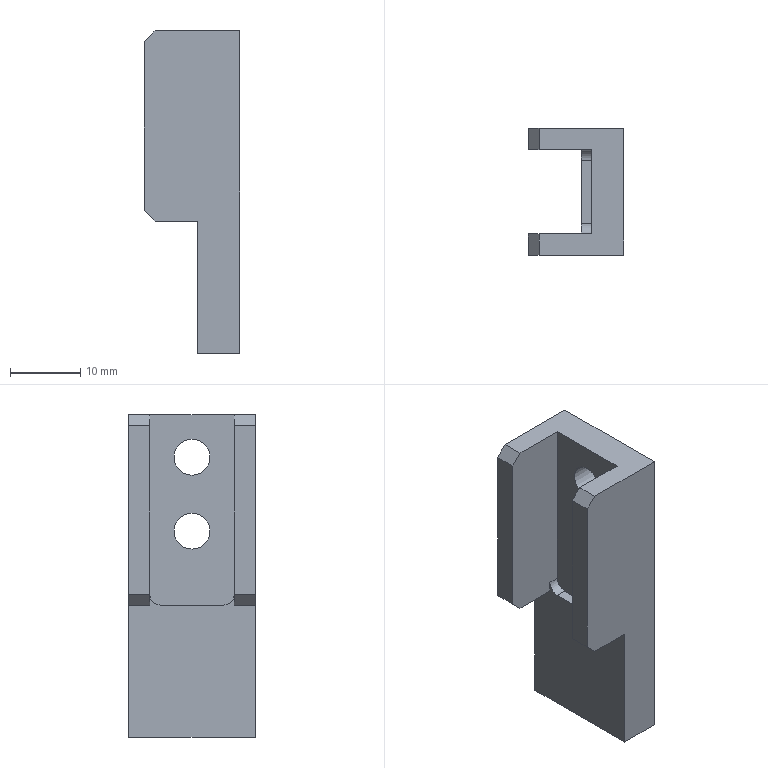Part | NX | features 倒角2 2 | 1 solid | 24 faces | box 13.5 x 18 x 45.75 mm | volume 5474 mm3 | plane 18 | cylinder 6 | commonest cylinder face diameters 5.1 x4 3 x2
STEP:
#1=CARTESIAN_POINT('',(126.798,-42.7,-33.95));
#2=VERTEX_POINT('',#1);
#3=CARTESIAN_POINT('',(126.798,-42.7,-39.05));
#4=VERTEX_POINT('',#3);
#5=CARTESIAN_POINT('',(126.798,-42.7,-36.5));
#6=DIRECTION('',(-1.,0.,0.));
#7=DIRECTION('',(0.,0.,1.));
#8=AXIS2_PLACEMENT_3D('',#5,#6,#7);
#9=CIRCLE('',#8,2.55);
#10=EDGE_CURVE('',#2,#4,#9,.F.);
#11=ORIENTED_EDGE('',*,*,#10,.F.);
#12=CARTESIAN_POINT('',(131.298,-42.7,-33.95));
#13=VERTEX_POINT('',#12);
#14=CARTESIAN_POINT('',(131.298,-42.7,-33.95));
#15=DIRECTION('',(1.,0.,0.));
#16=VECTOR('',#15,1000.);
#17=LINE('',#14,#16);
#18=EDGE_CURVE('',#13,#2,#17,.F.);
#19=ORIENTED_EDGE('',*,*,#18,.F.);
#20=CARTESIAN_POINT('',(131.298,-42.7,-39.05));
#21=VERTEX_POINT('',#20);
#22=CARTESIAN_POINT('',(131.298,-42.7,-36.5));
#23=DIRECTION('',(-1.,0.,0.));
#24=DIRECTION('',(0.,0.,1.));
#25=AXIS2_PLACEMENT_3D('',#22,#23,#24);
#26=CIRCLE('',#25,2.55);
#27=EDGE_CURVE('',#13,#21,#26,.F.);
#28=ORIENTED_EDGE('',*,*,#27,.T.);
#29=CARTESIAN_POINT('',(131.298,-42.7,-39.05));
#30=DIRECTION('',(1.,0.,0.));
#31=VECTOR('',#30,1000.);
#32=LINE('',#29,#31);
#33=EDGE_CURVE('',#4,#21,#32,.T.);
#34=ORIENTED_EDGE('',*,*,#33,.F.);
#35=EDGE_LOOP('',(#11,#19,#28,#34));
#36=FACE_BOUND('',#35,.T.);
#37=CARTESIAN_POINT('',(131.298,-42.7,-36.5));
#38=DIRECTION('',(1.,0.,0.));
#39=DIRECTION('',(0.,0.,-1.));
#40=AXIS2_PLACEMENT_3D('',#37,#38,#39);
#41=CYLINDRICAL_SURFACE('',#40,2.55);
#42=ADVANCED_FACE('',(#36),#41,.F.);
#43=CARTESIAN_POINT('',(126.798,-42.7,-23.45));
#44=VERTEX_POINT('',#43);
#45=CARTESIAN_POINT('',(126.798,-42.7,-28.55));
#46=VERTEX_POINT('',#45);
#47=CARTESIAN_POINT('',(126.798,-42.7,-26.));
#48=DIRECTION('',(-1.,0.,0.));
#49=DIRECTION('',(0.,0.,1.));
#50=AXIS2_PLACEMENT_3D('',#47,#48,#49);
#51=CIRCLE('',#50,2.55);
#52=EDGE_CURVE('',#44,#46,#51,.F.);
#53=ORIENTED_EDGE('',*,*,#52,.F.);
#54=CARTESIAN_POINT('',(131.298,-42.7,-23.45));
#55=VERTEX_POINT('',#54);
#56=CARTESIAN_POINT('',(131.298,-42.7,-23.45));
#57=DIRECTION('',(1.,0.,0.));
#58=VECTOR('',#57,1000.);
#59=LINE('',#56,#58);
#60=EDGE_CURVE('',#55,#44,#59,.F.);
#61=ORIENTED_EDGE('',*,*,#60,.F.);
#62=CARTESIAN_POINT('',(131.298,-42.7,-28.55));
#63=VERTEX_POINT('',#62);
#64=CARTESIAN_POINT('',(131.298,-42.7,-26.));
#65=DIRECTION('',(-1.,0.,0.));
#66=DIRECTION('',(0.,0.,1.));
#67=AXIS2_PLACEMENT_3D('',#64,#65,#66);
#68=CIRCLE('',#67,2.55);
#69=EDGE_CURVE('',#55,#63,#68,.F.);
#70=ORIENTED_EDGE('',*,*,#69,.T.);
#71=CARTESIAN_POINT('',(131.298,-42.7,-28.55));
#72=DIRECTION('',(1.,0.,0.));
#73=VECTOR('',#72,1000.);
#74=LINE('',#71,#73);
#75=EDGE_CURVE('',#46,#63,#74,.T.);
#76=ORIENTED_EDGE('',*,*,#75,.F.);
#77=EDGE_LOOP('',(#53,#61,#70,#76));
#78=FACE_BOUND('',#77,.T.);
#79=CARTESIAN_POINT('',(131.298,-42.7,-26.));
#80=DIRECTION('',(1.,0.,0.));
#81=DIRECTION('',(0.,0.,-1.));
#82=AXIS2_PLACEMENT_3D('',#79,#80,#81);
#83=CYLINDRICAL_SURFACE('',#82,2.55);
#84=ADVANCED_FACE('',(#78),#83,.F.);
#85=CARTESIAN_POINT('',(117.798,-33.7,-45.5));
#86=VERTEX_POINT('',#85);
#87=CARTESIAN_POINT('',(117.798,-33.7,-21.5));
#88=VERTEX_POINT('',#87);
#89=CARTESIAN_POINT('',(117.798,-33.7,-42.5));
#90=DIRECTION('',(0.,0.,-1.));
#91=VECTOR('',#90,1000.);
#92=LINE('',#89,#91);
#93=EDGE_CURVE('',#86,#88,#92,.F.);
#94=ORIENTED_EDGE('',*,*,#93,.F.);
#95=CARTESIAN_POINT('',(117.798,-36.7,-45.5));
#96=VERTEX_POINT('',#95);
#97=CARTESIAN_POINT('',(117.798,-33.7,-45.5));
#98=DIRECTION('',(0.,1.,0.));
#99=VECTOR('',#98,1000.);
#100=LINE('',#97,#99);
#101=EDGE_CURVE('',#86,#96,#100,.F.);
#102=ORIENTED_EDGE('',*,*,#101,.T.);
#103=CARTESIAN_POINT('',(117.798,-36.7,-21.5));
#104=VERTEX_POINT('',#103);
#105=CARTESIAN_POINT('',(117.798,-36.7,-20.));
#106=DIRECTION('',(0.,0.,1.));
#107=VECTOR('',#106,1000.);
#108=LINE('',#105,#107);
#109=EDGE_CURVE('',#104,#96,#108,.F.);
#110=ORIENTED_EDGE('',*,*,#109,.F.);
#111=CARTESIAN_POINT('',(117.798,-36.7,-21.5));
#112=DIRECTION('',(0.,-1.,0.));
#113=VECTOR('',#112,1000.);
#114=LINE('',#111,#113);
#115=EDGE_CURVE('',#104,#88,#114,.F.);
#116=ORIENTED_EDGE('',*,*,#115,.T.);
#117=EDGE_LOOP('',(#94,#102,#110,#116));
#118=FACE_BOUND('',#117,.T.);
#119=CARTESIAN_POINT('',(117.798,-42.7,-31.25));
#120=DIRECTION('',(-1.,0.,0.));
#121=DIRECTION('',(0.,0.,1.));
#122=AXIS2_PLACEMENT_3D('',#119,#120,#121);
#123=PLANE('',#122);
#124=ADVANCED_FACE('',(#118),#123,.T.);
#125=CARTESIAN_POINT('',(125.298,-33.7,-65.75));
#126=VERTEX_POINT('',#125);
#127=CARTESIAN_POINT('',(125.298,-51.7,-65.75));
#128=VERTEX_POINT('',#127);
#129=CARTESIAN_POINT('',(125.298,-51.7,-65.75));
#130=DIRECTION('',(0.,1.,0.));
#131=VECTOR('',#130,1000.);
#132=LINE('',#129,#131);
#133=EDGE_CURVE('',#126,#128,#132,.F.);
#134=ORIENTED_EDGE('',*,*,#133,.F.);
#135=CARTESIAN_POINT('',(131.298,-33.7,-65.75));
#136=VERTEX_POINT('',#135);
#137=CARTESIAN_POINT('',(88.395,-33.7,-65.75));
#138=DIRECTION('',(-1.,0.,0.));
#139=VECTOR('',#138,1000.);
#140=LINE('',#137,#139);
#141=EDGE_CURVE('',#136,#126,#140,.T.);
#142=ORIENTED_EDGE('',*,*,#141,.F.);
#143=CARTESIAN_POINT('',(131.298,-51.7,-65.75));
#144=VERTEX_POINT('',#143);
#145=CARTESIAN_POINT('',(131.298,-33.7,-65.75));
#146=DIRECTION('',(0.,-1.,0.));
#147=VECTOR('',#146,1000.);
#148=LINE('',#145,#147);
#149=EDGE_CURVE('',#144,#136,#148,.F.);
#150=ORIENTED_EDGE('',*,*,#149,.F.);
#151=CARTESIAN_POINT('',(131.298,-51.7,-65.75));
#152=DIRECTION('',(-1.,0.,0.));
#153=VECTOR('',#152,1000.);
#154=LINE('',#151,#153);
#155=EDGE_CURVE('',#144,#128,#154,.T.);
#156=ORIENTED_EDGE('',*,*,#155,.T.);
#157=EDGE_LOOP('',(#134,#142,#150,#156));
#158=FACE_BOUND('',#157,.T.);
#159=CARTESIAN_POINT('',(88.395,-33.7,-65.75));
#160=DIRECTION('',(0.,0.,-1.));
#161=DIRECTION('',(-1.,0.,0.));
#162=AXIS2_PLACEMENT_3D('',#159,#160,#161);
#163=PLANE('',#162);
#164=ADVANCED_FACE('',(#158),#163,.T.);
#165=CARTESIAN_POINT('',(125.298,-47.2,-47.));
#166=VERTEX_POINT('',#165);
#167=CARTESIAN_POINT('',(125.298,-38.2,-47.));
#168=VERTEX_POINT('',#167);
#169=CARTESIAN_POINT('',(125.298,-51.7,-47.));
#170=DIRECTION('',(0.,-1.,0.));
#171=VECTOR('',#170,1000.);
#172=LINE('',#169,#171);
#173=EDGE_CURVE('',#166,#168,#172,.F.);
#174=ORIENTED_EDGE('',*,*,#173,.F.);
#175=CARTESIAN_POINT('',(126.798,-47.2,-47.));
#176=VERTEX_POINT('',#175);
#177=CARTESIAN_POINT('',(125.298,-47.2,-47.));
#178=DIRECTION('',(-1.,0.,0.));
#179=VECTOR('',#178,1000.);
#180=LINE('',#177,#179);
#181=EDGE_CURVE('',#166,#176,#180,.F.);
#182=ORIENTED_EDGE('',*,*,#181,.T.);
#183=CARTESIAN_POINT('',(126.798,-38.2,-47.));
#184=VERTEX_POINT('',#183);
#185=CARTESIAN_POINT('',(126.798,-48.7,-47.));
#186=DIRECTION('',(0.,1.,0.));
#187=VECTOR('',#186,1000.);
#188=LINE('',#185,#187);
#189=EDGE_CURVE('',#184,#176,#188,.F.);
#190=ORIENTED_EDGE('',*,*,#189,.F.);
#191=CARTESIAN_POINT('',(126.798,-38.2,-47.));
#192=DIRECTION('',(1.,0.,0.));
#193=VECTOR('',#192,1000.);
#194=LINE('',#191,#193);
#195=EDGE_CURVE('',#184,#168,#194,.F.);
#196=ORIENTED_EDGE('',*,*,#195,.T.);
#197=EDGE_LOOP('',(#174,#182,#190,#196));
#198=FACE_BOUND('',#197,.T.);
#199=CARTESIAN_POINT('',(126.798,-48.7,-47.));
#200=DIRECTION('',(0.,0.,-1.));
#201=DIRECTION('',(0.,1.,0.));
#202=AXIS2_PLACEMENT_3D('',#199,#200,#201);
#203=PLANE('',#202);
#204=ADVANCED_FACE('',(#198),#203,.F.);
#205=CARTESIAN_POINT('',(119.298,-36.7,-20.));
#206=VERTEX_POINT('',#205);
#207=CARTESIAN_POINT('',(126.798,-36.7,-20.));
#208=VERTEX_POINT('',#207);
#209=CARTESIAN_POINT('',(126.798,-36.7,-20.));
#210=DIRECTION('',(-1.,0.,0.));
#211=VECTOR('',#210,1000.);
#212=LINE('',#209,#211);
#213=EDGE_CURVE('',#206,#208,#212,.F.);
#214=ORIENTED_EDGE('',*,*,#213,.T.);
#215=CARTESIAN_POINT('',(126.798,-48.7,-20.));
#216=VERTEX_POINT('',#215);
#217=CARTESIAN_POINT('',(126.798,-48.7,-20.));
#218=DIRECTION('',(0.,-1.,0.));
#219=VECTOR('',#218,1000.);
#220=LINE('',#217,#219);
#221=EDGE_CURVE('',#216,#208,#220,.F.);
#222=ORIENTED_EDGE('',*,*,#221,.F.);
#223=CARTESIAN_POINT('',(119.298,-48.7,-20.));
#224=VERTEX_POINT('',#223);
#225=CARTESIAN_POINT('',(126.798,-48.7,-20.));
#226=DIRECTION('',(-1.,0.,0.));
#227=VECTOR('',#226,1000.);
#228=LINE('',#225,#227);
#229=EDGE_CURVE('',#224,#216,#228,.F.);
#230=ORIENTED_EDGE('',*,*,#229,.F.);
#231=CARTESIAN_POINT('',(119.298,-51.7,-20.));
#232=VERTEX_POINT('',#231);
#233=CARTESIAN_POINT('',(119.298,-48.7,-20.));
#234=DIRECTION('',(0.,1.,0.));
#235=VECTOR('',#234,1000.);
#236=LINE('',#233,#235);
#237=EDGE_CURVE('',#224,#232,#236,.F.);
#238=ORIENTED_EDGE('',*,*,#237,.T.);
#239=CARTESIAN_POINT('',(131.298,-51.7,-20.));
#240=VERTEX_POINT('',#239);
#241=CARTESIAN_POINT('',(131.298,-51.7,-20.));
#242=DIRECTION('',(-1.,0.,0.));
#243=VECTOR('',#242,1000.);
#244=LINE('',#241,#243);
#245=EDGE_CURVE('',#232,#240,#244,.F.);
#246=ORIENTED_EDGE('',*,*,#245,.T.);
#247=CARTESIAN_POINT('',(131.298,-33.7,-20.));
#248=VERTEX_POINT('',#247);
#249=CARTESIAN_POINT('',(131.298,-51.7,-20.));
#250=DIRECTION('',(0.,1.,0.));
#251=VECTOR('',#250,1000.);
#252=LINE('',#249,#251);
#253=EDGE_CURVE('',#248,#240,#252,.F.);
#254=ORIENTED_EDGE('',*,*,#253,.F.);
#255=CARTESIAN_POINT('',(119.298,-33.7,-20.));
#256=VERTEX_POINT('',#255);
#257=CARTESIAN_POINT('',(131.298,-33.7,-20.));
#258=DIRECTION('',(-1.,0.,0.));
#259=VECTOR('',#258,1000.);
#260=LINE('',#257,#259);
#261=EDGE_CURVE('',#256,#248,#260,.F.);
#262=ORIENTED_EDGE('',*,*,#261,.F.);
#263=CARTESIAN_POINT('',(119.298,-33.7,-20.));
#264=DIRECTION('',(0.,1.,0.));
#265=VECTOR('',#264,1000.);
#266=LINE('',#263,#265);
#267=EDGE_CURVE('',#256,#206,#266,.F.);
#268=ORIENTED_EDGE('',*,*,#267,.T.);
#269=EDGE_LOOP('',(#214,#222,#230,#238,#246,#254,#262,#268));
#270=FACE_BOUND('',#269,.T.);
#271=CARTESIAN_POINT('',(131.298,-51.7,-20.));
#272=DIRECTION('',(0.,0.,-1.));
#273=DIRECTION('',(-1.,0.,0.));
#274=AXIS2_PLACEMENT_3D('',#271,#272,#273);
#275=PLANE('',#274);
#276=ADVANCED_FACE('',(#270),#275,.F.);
#277=ORIENTED_EDGE('',*,*,#261,.T.);
#278=CARTESIAN_POINT('',(131.298,-33.7,-42.5));
#279=DIRECTION('',(0.,0.,-1.));
#280=VECTOR('',#279,1000.);
#281=LINE('',#278,#280);
#282=EDGE_CURVE('',#136,#248,#281,.F.);
#283=ORIENTED_EDGE('',*,*,#282,.F.);
#284=ORIENTED_EDGE('',*,*,#141,.T.);
#285=CARTESIAN_POINT('',(125.298,-33.7,-47.));
#286=VERTEX_POINT('',#285);
#287=CARTESIAN_POINT('',(125.298,-33.7,-65.75));
#288=DIRECTION('',(0.,0.,1.));
#289=VECTOR('',#288,1000.);
#290=LINE('',#287,#289);
#291=EDGE_CURVE('',#286,#126,#290,.F.);
#292=ORIENTED_EDGE('',*,*,#291,.F.);
#293=CARTESIAN_POINT('',(119.298,-33.7,-47.));
#294=VERTEX_POINT('',#293);
#295=CARTESIAN_POINT('',(125.298,-33.7,-47.));
#296=DIRECTION('',(-1.,0.,0.));
#297=VECTOR('',#296,1000.);
#298=LINE('',#295,#297);
#299=EDGE_CURVE('',#294,#286,#298,.F.);
#300=ORIENTED_EDGE('',*,*,#299,.F.);
#301=CARTESIAN_POINT('',(119.298,-33.7,-47.));
#302=DIRECTION('',(0.7071,0.,-0.7071));
#303=VECTOR('',#302,1000.);
#304=LINE('',#301,#303);
#305=EDGE_CURVE('',#294,#86,#304,.F.);
#306=ORIENTED_EDGE('',*,*,#305,.T.);
#307=ORIENTED_EDGE('',*,*,#93,.T.);
#308=CARTESIAN_POINT('',(119.298,-33.7,-20.));
#309=DIRECTION('',(-0.7071,0.,-0.7071));
#310=VECTOR('',#309,1000.);
#311=LINE('',#308,#310);
#312=EDGE_CURVE('',#88,#256,#311,.F.);
#313=ORIENTED_EDGE('',*,*,#312,.T.);
#314=EDGE_LOOP('',(#277,#283,#284,#292,#300,#306,#307,#313));
#315=FACE_BOUND('',#314,.T.);
#316=CARTESIAN_POINT('',(131.298,-33.7,-42.5));
#317=DIRECTION('',(0.,-1.,0.));
#318=DIRECTION('',(1.,0.,0.));
#319=AXIS2_PLACEMENT_3D('',#316,#317,#318);
#320=PLANE('',#319);
#321=ADVANCED_FACE('',(#315),#320,.F.);
#322=CARTESIAN_POINT('',(117.798,-51.7,-21.5));
#323=VERTEX_POINT('',#322);
#324=CARTESIAN_POINT('',(117.798,-51.7,-45.5));
#325=VERTEX_POINT('',#324);
#326=CARTESIAN_POINT('',(117.798,-51.7,-42.5));
#327=DIRECTION('',(0.,0.,1.));
#328=VECTOR('',#327,1000.);
#329=LINE('',#326,#328);
#330=EDGE_CURVE('',#323,#325,#329,.F.);
#331=ORIENTED_EDGE('',*,*,#330,.T.);
#332=CARTESIAN_POINT('',(119.298,-51.7,-47.));
#333=VERTEX_POINT('',#332);
#334=CARTESIAN_POINT('',(119.298,-51.7,-47.));
#335=DIRECTION('',(-0.7071,0.,0.7071));
#336=VECTOR('',#335,1000.);
#337=LINE('',#334,#336);
#338=EDGE_CURVE('',#325,#333,#337,.F.);
#339=ORIENTED_EDGE('',*,*,#338,.T.);
#340=CARTESIAN_POINT('',(125.298,-51.7,-47.));
#341=VERTEX_POINT('',#340);
#342=CARTESIAN_POINT('',(125.298,-51.7,-47.));
#343=DIRECTION('',(-1.,0.,0.));
#344=VECTOR('',#343,1000.);
#345=LINE('',#342,#344);
#346=EDGE_CURVE('',#333,#341,#345,.F.);
#347=ORIENTED_EDGE('',*,*,#346,.T.);
#348=CARTESIAN_POINT('',(125.298,-51.7,-65.75));
#349=DIRECTION('',(0.,0.,-1.));
#350=VECTOR('',#349,1000.);
#351=LINE('',#348,#350);
#352=EDGE_CURVE('',#128,#341,#351,.F.);
#353=ORIENTED_EDGE('',*,*,#352,.F.);
#354=ORIENTED_EDGE('',*,*,#155,.F.);
#355=CARTESIAN_POINT('',(131.298,-51.7,-42.5));
#356=DIRECTION('',(0.,0.,1.));
#357=VECTOR('',#356,1000.);
#358=LINE('',#355,#357);
#359=EDGE_CURVE('',#240,#144,#358,.F.);
#360=ORIENTED_EDGE('',*,*,#359,.F.);
#361=ORIENTED_EDGE('',*,*,#245,.F.);
#362=CARTESIAN_POINT('',(119.298,-51.7,-20.));
#363=DIRECTION('',(0.7071,0.,0.7071));
#364=VECTOR('',#363,1000.);
#365=LINE('',#362,#364);
#366=EDGE_CURVE('',#232,#323,#365,.F.);
#367=ORIENTED_EDGE('',*,*,#366,.T.);
#368=EDGE_LOOP('',(#331,#339,#347,#353,#354,#360,#361,#367));
#369=FACE_BOUND('',#368,.T.);
#370=CARTESIAN_POINT('',(131.298,-51.7,-42.5));
#371=DIRECTION('',(0.,1.,0.));
#372=DIRECTION('',(-1.,0.,0.));
#373=AXIS2_PLACEMENT_3D('',#370,#371,#372);
#374=PLANE('',#373);
#375=ADVANCED_FACE('',(#369),#374,.F.);
#376=CARTESIAN_POINT('',(131.298,-42.7,-36.5));
#377=DIRECTION('',(-1.,0.,0.));
#378=DIRECTION('',(0.,0.,1.));
#379=AXIS2_PLACEMENT_3D('',#376,#377,#378);
#380=CIRCLE('',#379,2.55);
#381=EDGE_CURVE('',#21,#13,#380,.F.);
#382=ORIENTED_EDGE('',*,*,#381,.F.);
#383=ORIENTED_EDGE('',*,*,#27,.F.);
#384=EDGE_LOOP('',(#382,#383));
#385=FACE_BOUND('',#384,.T.);
#386=CARTESIAN_POINT('',(131.298,-42.7,-26.));
#387=DIRECTION('',(-1.,0.,0.));
#388=DIRECTION('',(0.,0.,1.));
#389=AXIS2_PLACEMENT_3D('',#386,#387,#388);
#390=CIRCLE('',#389,2.55);
#391=EDGE_CURVE('',#63,#55,#390,.F.);
#392=ORIENTED_EDGE('',*,*,#391,.F.);
#393=ORIENTED_EDGE('',*,*,#69,.F.);
#394=EDGE_LOOP('',(#392,#393));
#395=FACE_BOUND('',#394,.T.);
#396=ORIENTED_EDGE('',*,*,#149,.T.);
#397=ORIENTED_EDGE('',*,*,#282,.T.);
#398=ORIENTED_EDGE('',*,*,#253,.T.);
#399=ORIENTED_EDGE('',*,*,#359,.T.);
#400=EDGE_LOOP('',(#396,#397,#398,#399));
#401=FACE_BOUND('',#400,.T.);
#402=CARTESIAN_POINT('',(131.298,-42.7,-31.25));
#403=DIRECTION('',(-1.,0.,0.));
#404=DIRECTION('',(0.,0.,1.));
#405=AXIS2_PLACEMENT_3D('',#402,#403,#404);
#406=PLANE('',#405);
#407=ADVANCED_FACE('',(#385,#395,#401),#406,.F.);
#408=CARTESIAN_POINT('',(117.798,-48.7,-45.5));
#409=VERTEX_POINT('',#408);
#410=CARTESIAN_POINT('',(117.798,-48.7,-21.5));
#411=VERTEX_POINT('',#410);
#412=CARTESIAN_POINT('',(117.798,-48.7,-20.));
#413=DIRECTION('',(0.,0.,-1.));
#414=VECTOR('',#413,1000.);
#415=LINE('',#412,#414);
#416=EDGE_CURVE('',#409,#411,#415,.F.);
#417=ORIENTED_EDGE('',*,*,#416,.F.);
#418=CARTESIAN_POINT('',(117.798,-48.7,-45.5));
#419=DIRECTION('',(0.,1.,0.));
#420=VECTOR('',#419,1000.);
#421=LINE('',#418,#420);
#422=EDGE_CURVE('',#409,#325,#421,.F.);
#423=ORIENTED_EDGE('',*,*,#422,.T.);
#424=ORIENTED_EDGE('',*,*,#330,.F.);
#425=CARTESIAN_POINT('',(117.798,-51.7,-21.5));
#426=DIRECTION('',(0.,-1.,0.));
#427=VECTOR('',#426,1000.);
#428=LINE('',#425,#427);
#429=EDGE_CURVE('',#323,#411,#428,.F.);
#430=ORIENTED_EDGE('',*,*,#429,.T.);
#431=EDGE_LOOP('',(#417,#423,#424,#430));
#432=FACE_BOUND('',#431,.T.);
#433=CARTESIAN_POINT('',(117.798,-42.7,-31.25));
#434=DIRECTION('',(-1.,0.,0.));
#435=DIRECTION('',(0.,0.,1.));
#436=AXIS2_PLACEMENT_3D('',#433,#434,#435);
#437=PLANE('',#436);
#438=ADVANCED_FACE('',(#432),#437,.T.);
#439=ORIENTED_EDGE('',*,*,#109,.T.);
#440=CARTESIAN_POINT('',(119.298,-36.7,-47.));
#441=VERTEX_POINT('',#440);
#442=CARTESIAN_POINT('',(119.298,-36.7,-47.));
#443=DIRECTION('',(-0.7071,0.,0.7071));
#444=VECTOR('',#443,1000.);
#445=LINE('',#442,#444);
#446=EDGE_CURVE('',#96,#441,#445,.F.);
#447=ORIENTED_EDGE('',*,*,#446,.T.);
#448=CARTESIAN_POINT('',(125.298,-36.7,-47.));
#449=VERTEX_POINT('',#448);
#450=CARTESIAN_POINT('',(126.798,-36.7,-47.));
#451=DIRECTION('',(-1.,0.,0.));
#452=VECTOR('',#451,1000.);
#453=LINE('',#450,#452);
#454=EDGE_CURVE('',#441,#449,#453,.F.);
#455=ORIENTED_EDGE('',*,*,#454,.T.);
#456=CARTESIAN_POINT('',(125.298,-36.7,-45.5));
#457=VERTEX_POINT('',#456);
#458=CARTESIAN_POINT('',(125.298,-36.7,-20.));
#459=DIRECTION('',(0.,0.,-1.));
#460=VECTOR('',#459,1000.);
#461=LINE('',#458,#460);
#462=EDGE_CURVE('',#449,#457,#461,.F.);
#463=ORIENTED_EDGE('',*,*,#462,.T.);
#464=CARTESIAN_POINT('',(126.798,-36.7,-45.5));
#465=VERTEX_POINT('',#464);
#466=CARTESIAN_POINT('',(125.298,-36.7,-45.5));
#467=DIRECTION('',(-1.,0.,0.));
#468=VECTOR('',#467,1000.);
#469=LINE('',#466,#468);
#470=EDGE_CURVE('',#457,#465,#469,.F.);
#471=ORIENTED_EDGE('',*,*,#470,.T.);
#472=CARTESIAN_POINT('',(126.798,-36.7,-20.));
#473=DIRECTION('',(0.,0.,1.));
#474=VECTOR('',#473,1000.);
#475=LINE('',#472,#474);
#476=EDGE_CURVE('',#208,#465,#475,.F.);
#477=ORIENTED_EDGE('',*,*,#476,.F.);
#478=ORIENTED_EDGE('',*,*,#213,.F.);
#479=CARTESIAN_POINT('',(119.298,-36.7,-20.));
#480=DIRECTION('',(0.7071,0.,0.7071));
#481=VECTOR('',#480,1000.);
#482=LINE('',#479,#481);
#483=EDGE_CURVE('',#206,#104,#482,.F.);
#484=ORIENTED_EDGE('',*,*,#483,.T.);
#485=EDGE_LOOP('',(#439,#447,#455,#463,#471,#477,#478,#484));
#486=FACE_BOUND('',#485,.T.);
#487=CARTESIAN_POINT('',(126.798,-36.7,-20.));
#488=DIRECTION('',(0.,1.,0.));
#489=DIRECTION('',(-1.,0.,0.));
#490=AXIS2_PLACEMENT_3D('',#487,#488,#489);
#491=PLANE('',#490);
#492=ADVANCED_FACE('',(#486),#491,.F.);
#493=ORIENTED_EDGE('',*,*,#229,.T.);
#494=CARTESIAN_POINT('',(126.798,-48.7,-45.5));
#495=VERTEX_POINT('',#494);
#496=CARTESIAN_POINT('',(126.798,-48.7,-20.));
#497=DIRECTION('',(0.,0.,-1.));
#498=VECTOR('',#497,1000.);
#499=LINE('',#496,#498);
#500=EDGE_CURVE('',#495,#216,#499,.F.);
#501=ORIENTED_EDGE('',*,*,#500,.F.);
#502=CARTESIAN_POINT('',(125.298,-48.7,-45.5));
#503=VERTEX_POINT('',#502);
#504=CARTESIAN_POINT('',(126.798,-48.7,-45.5));
#505=DIRECTION('',(1.,0.,0.));
#506=VECTOR('',#505,1000.);
#507=LINE('',#504,#506);
#508=EDGE_CURVE('',#495,#503,#507,.F.);
#509=ORIENTED_EDGE('',*,*,#508,.T.);
#510=CARTESIAN_POINT('',(125.298,-48.7,-47.));
#511=VERTEX_POINT('',#510);
#512=CARTESIAN_POINT('',(125.298,-48.7,-20.));
#513=DIRECTION('',(0.,0.,1.));
#514=VECTOR('',#513,1000.);
#515=LINE('',#512,#514);
#516=EDGE_CURVE('',#503,#511,#515,.F.);
#517=ORIENTED_EDGE('',*,*,#516,.T.);
#518=CARTESIAN_POINT('',(119.298,-48.7,-47.));
#519=VERTEX_POINT('',#518);
#520=CARTESIAN_POINT('',(126.798,-48.7,-47.));
#521=DIRECTION('',(-1.,0.,0.));
#522=VECTOR('',#521,1000.);
#523=LINE('',#520,#522);
#524=EDGE_CURVE('',#519,#511,#523,.F.);
#525=ORIENTED_EDGE('',*,*,#524,.F.);
#526=CARTESIAN_POINT('',(119.298,-48.7,-47.));
#527=DIRECTION('',(0.7071,0.,-0.7071));
#528=VECTOR('',#527,1000.);
#529=LINE('',#526,#528);
#530=EDGE_CURVE('',#519,#409,#529,.F.);
#531=ORIENTED_EDGE('',*,*,#530,.T.);
#532=ORIENTED_EDGE('',*,*,#416,.T.);
#533=CARTESIAN_POINT('',(119.298,-48.7,-20.));
#534=DIRECTION('',(-0.7071,0.,-0.7071));
#535=VECTOR('',#534,1000.);
#536=LINE('',#533,#535);
#537=EDGE_CURVE('',#411,#224,#536,.F.);
#538=ORIENTED_EDGE('',*,*,#537,.T.);
#539=EDGE_LOOP('',(#493,#501,#509,#517,#525,#531,#532,#538));
#540=FACE_BOUND('',#539,.T.);
#541=CARTESIAN_POINT('',(126.798,-48.7,-20.));
#542=DIRECTION('',(0.,-1.,0.));
#543=DIRECTION('',(0.,0.,-1.));
#544=AXIS2_PLACEMENT_3D('',#541,#542,#543);
#545=PLANE('',#544);
#546=ADVANCED_FACE('',(#540),#545,.F.);
#547=CARTESIAN_POINT('',(126.798,-42.7,-36.5));
#548=DIRECTION('',(-1.,0.,0.));
#549=DIRECTION('',(0.,0.,1.));
#550=AXIS2_PLACEMENT_3D('',#547,#548,#549);
#551=CIRCLE('',#550,2.55);
#552=EDGE_CURVE('',#4,#2,#551,.F.);
#553=ORIENTED_EDGE('',*,*,#552,.T.);
#554=ORIENTED_EDGE('',*,*,#10,.T.);
#555=EDGE_LOOP('',(#553,#554));
#556=FACE_BOUND('',#555,.T.);
#557=CARTESIAN_POINT('',(126.798,-42.7,-26.));
#558=DIRECTION('',(-1.,0.,0.));
#559=DIRECTION('',(0.,0.,1.));
#560=AXIS2_PLACEMENT_3D('',#557,#558,#559);
#561=CIRCLE('',#560,2.55);
#562=EDGE_CURVE('',#46,#44,#561,.F.);
#563=ORIENTED_EDGE('',*,*,#562,.T.);
#564=ORIENTED_EDGE('',*,*,#52,.T.);
#565=EDGE_LOOP('',(#563,#564));
#566=FACE_BOUND('',#565,.T.);
#567=ORIENTED_EDGE('',*,*,#189,.T.);
#568=CARTESIAN_POINT('',(126.798,-47.2,-45.5));
#569=DIRECTION('',(1.,0.,0.));
#570=DIRECTION('',(0.,0.,1.));
#571=AXIS2_PLACEMENT_3D('',#568,#569,#570);
#572=CIRCLE('',#571,1.5);
#573=EDGE_CURVE('',#176,#495,#572,.F.);
#574=ORIENTED_EDGE('',*,*,#573,.T.);
#575=ORIENTED_EDGE('',*,*,#500,.T.);
#576=ORIENTED_EDGE('',*,*,#221,.T.);
#577=ORIENTED_EDGE('',*,*,#476,.T.);
#578=CARTESIAN_POINT('',(126.798,-38.2,-45.5));
#579=DIRECTION('',(1.,0.,0.));
#580=DIRECTION('',(0.,0.,1.));
#581=AXIS2_PLACEMENT_3D('',#578,#579,#580);
#582=CIRCLE('',#581,1.5);
#583=EDGE_CURVE('',#465,#184,#582,.F.);
#584=ORIENTED_EDGE('',*,*,#583,.T.);
#585=EDGE_LOOP('',(#567,#574,#575,#576,#577,#584));
#586=FACE_BOUND('',#585,.T.);
#587=CARTESIAN_POINT('',(126.798,-42.7,-31.25));
#588=DIRECTION('',(1.,0.,0.));
#589=DIRECTION('',(0.,0.,-1.));
#590=AXIS2_PLACEMENT_3D('',#587,#588,#589);
#591=PLANE('',#590);
#592=ADVANCED_FACE('',(#556,#566,#586),#591,.F.);
#593=ORIENTED_EDGE('',*,*,#75,.T.);
#594=ORIENTED_EDGE('',*,*,#391,.T.);
#595=ORIENTED_EDGE('',*,*,#60,.T.);
#596=ORIENTED_EDGE('',*,*,#562,.F.);
#597=EDGE_LOOP('',(#593,#594,#595,#596));
#598=FACE_BOUND('',#597,.T.);
#599=CARTESIAN_POINT('',(131.298,-42.7,-26.));
#600=DIRECTION('',(1.,0.,0.));
#601=DIRECTION('',(0.,0.,-1.));
#602=AXIS2_PLACEMENT_3D('',#599,#600,#601);
#603=CYLINDRICAL_SURFACE('',#602,2.55);
#604=ADVANCED_FACE('',(#598),#603,.F.);
#605=ORIENTED_EDGE('',*,*,#33,.T.);
#606=ORIENTED_EDGE('',*,*,#381,.T.);
#607=ORIENTED_EDGE('',*,*,#18,.T.);
#608=ORIENTED_EDGE('',*,*,#552,.F.);
#609=EDGE_LOOP('',(#605,#606,#607,#608));
#610=FACE_BOUND('',#609,.T.);
#611=CARTESIAN_POINT('',(131.298,-42.7,-36.5));
#612=DIRECTION('',(1.,0.,0.));
#613=DIRECTION('',(0.,0.,-1.));
#614=AXIS2_PLACEMENT_3D('',#611,#612,#613);
#615=CYLINDRICAL_SURFACE('',#614,2.55);
#616=ADVANCED_FACE('',(#610),#615,.F.);
#617=ORIENTED_EDGE('',*,*,#299,.T.);
#618=CARTESIAN_POINT('',(125.298,-51.7,-47.));
#619=DIRECTION('',(0.,-1.,0.));
#620=VECTOR('',#619,1000.);
#621=LINE('',#618,#620);
#622=EDGE_CURVE('',#449,#286,#621,.F.);
#623=ORIENTED_EDGE('',*,*,#622,.F.);
#624=ORIENTED_EDGE('',*,*,#454,.F.);
#625=CARTESIAN_POINT('',(119.298,-36.7,-47.));
#626=DIRECTION('',(0.,-1.,0.));
#627=VECTOR('',#626,1000.);
#628=LINE('',#625,#627);
#629=EDGE_CURVE('',#441,#294,#628,.F.);
#630=ORIENTED_EDGE('',*,*,#629,.T.);
#631=EDGE_LOOP('',(#617,#623,#624,#630));
#632=FACE_BOUND('',#631,.T.);
#633=CARTESIAN_POINT('',(125.298,-51.7,-47.));
#634=DIRECTION('',(0.,0.,1.));
#635=DIRECTION('',(0.,-1.,0.));
#636=AXIS2_PLACEMENT_3D('',#633,#634,#635);
#637=PLANE('',#636);
#638=ADVANCED_FACE('',(#632),#637,.F.);
#639=ORIENTED_EDGE('',*,*,#524,.T.);
#640=CARTESIAN_POINT('',(125.298,-51.7,-47.));
#641=DIRECTION('',(0.,-1.,0.));
#642=VECTOR('',#641,1000.);
#643=LINE('',#640,#642);
#644=EDGE_CURVE('',#341,#511,#643,.F.);
#645=ORIENTED_EDGE('',*,*,#644,.F.);
#646=ORIENTED_EDGE('',*,*,#346,.F.);
#647=CARTESIAN_POINT('',(119.298,-51.7,-47.));
#648=DIRECTION('',(0.,-1.,0.));
#649=VECTOR('',#648,1000.);
#650=LINE('',#647,#649);
#651=EDGE_CURVE('',#333,#519,#650,.F.);
#652=ORIENTED_EDGE('',*,*,#651,.T.);
#653=EDGE_LOOP('',(#639,#645,#646,#652));
#654=FACE_BOUND('',#653,.T.);
#655=CARTESIAN_POINT('',(125.298,-51.7,-47.));
#656=DIRECTION('',(0.,0.,1.));
#657=DIRECTION('',(0.,-1.,0.));
#658=AXIS2_PLACEMENT_3D('',#655,#656,#657);
#659=PLANE('',#658);
#660=ADVANCED_FACE('',(#654),#659,.F.);
#661=ORIENTED_EDGE('',*,*,#352,.T.);
#662=ORIENTED_EDGE('',*,*,#644,.T.);
#663=ORIENTED_EDGE('',*,*,#516,.F.);
#664=CARTESIAN_POINT('',(125.298,-47.2,-45.5));
#665=DIRECTION('',(-1.,0.,0.));
#666=DIRECTION('',(0.,0.,-1.));
#667=AXIS2_PLACEMENT_3D('',#664,#665,#666);
#668=CIRCLE('',#667,1.5);
#669=EDGE_CURVE('',#503,#166,#668,.F.);
#670=ORIENTED_EDGE('',*,*,#669,.T.);
#671=ORIENTED_EDGE('',*,*,#173,.T.);
#672=CARTESIAN_POINT('',(125.298,-38.2,-45.5));
#673=DIRECTION('',(-1.,0.,0.));
#674=DIRECTION('',(0.,0.,-1.));
#675=AXIS2_PLACEMENT_3D('',#672,#673,#674);
#676=CIRCLE('',#675,1.5);
#677=EDGE_CURVE('',#168,#457,#676,.F.);
#678=ORIENTED_EDGE('',*,*,#677,.T.);
#679=ORIENTED_EDGE('',*,*,#462,.F.);
#680=ORIENTED_EDGE('',*,*,#622,.T.);
#681=ORIENTED_EDGE('',*,*,#291,.T.);
#682=ORIENTED_EDGE('',*,*,#133,.T.);
#683=EDGE_LOOP('',(#661,#662,#663,#670,#671,#678,#679,#680,#681,#682));
#684=FACE_BOUND('',#683,.T.);
#685=CARTESIAN_POINT('',(125.298,-42.7,-31.25));
#686=DIRECTION('',(-1.,0.,0.));
#687=DIRECTION('',(0.,0.,1.));
#688=AXIS2_PLACEMENT_3D('',#685,#686,#687);
#689=PLANE('',#688);
#690=ADVANCED_FACE('',(#684),#689,.T.);
#691=ORIENTED_EDGE('',*,*,#583,.F.);
#692=ORIENTED_EDGE('',*,*,#470,.F.);
#693=ORIENTED_EDGE('',*,*,#677,.F.);
#694=ORIENTED_EDGE('',*,*,#195,.F.);
#695=EDGE_LOOP('',(#691,#692,#693,#694));
#696=FACE_BOUND('',#695,.T.);
#697=CARTESIAN_POINT('',(126.798,-38.2,-45.5));
#698=DIRECTION('',(1.,0.,0.));
#699=DIRECTION('',(0.,0.,-1.));
#700=AXIS2_PLACEMENT_3D('',#697,#698,#699);
#701=CYLINDRICAL_SURFACE('',#700,1.5);
#702=ADVANCED_FACE('',(#696),#701,.F.);
#703=ORIENTED_EDGE('',*,*,#573,.F.);
#704=ORIENTED_EDGE('',*,*,#181,.F.);
#705=ORIENTED_EDGE('',*,*,#669,.F.);
#706=ORIENTED_EDGE('',*,*,#508,.F.);
#707=EDGE_LOOP('',(#703,#704,#705,#706));
#708=FACE_BOUND('',#707,.T.);
#709=CARTESIAN_POINT('',(126.798,-47.2,-45.5));
#710=DIRECTION('',(1.,0.,0.));
#711=DIRECTION('',(0.,0.,-1.));
#712=AXIS2_PLACEMENT_3D('',#709,#710,#711);
#713=CYLINDRICAL_SURFACE('',#712,1.5);
#714=ADVANCED_FACE('',(#708),#713,.F.);
#715=ORIENTED_EDGE('',*,*,#483,.F.);
#716=ORIENTED_EDGE('',*,*,#267,.F.);
#717=ORIENTED_EDGE('',*,*,#312,.F.);
#718=ORIENTED_EDGE('',*,*,#115,.F.);
#719=EDGE_LOOP('',(#715,#716,#717,#718));
#720=FACE_BOUND('',#719,.T.);
#721=CARTESIAN_POINT('',(119.298,-51.7,-20.));
#722=DIRECTION('',(-0.7071,0.,0.7071));
#723=DIRECTION('',(0.,1.,0.));
#724=AXIS2_PLACEMENT_3D('',#721,#722,#723);
#725=PLANE('',#724);
#726=ADVANCED_FACE('',(#720),#725,.T.);
#727=ORIENTED_EDGE('',*,*,#366,.F.);
#728=ORIENTED_EDGE('',*,*,#237,.F.);
#729=ORIENTED_EDGE('',*,*,#537,.F.);
#730=ORIENTED_EDGE('',*,*,#429,.F.);
#731=EDGE_LOOP('',(#727,#728,#729,#730));
#732=FACE_BOUND('',#731,.T.);
#733=CARTESIAN_POINT('',(119.298,-51.7,-20.));
#734=DIRECTION('',(-0.7071,0.,0.7071));
#735=DIRECTION('',(0.,1.,0.));
#736=AXIS2_PLACEMENT_3D('',#733,#734,#735);
#737=PLANE('',#736);
#738=ADVANCED_FACE('',(#732),#737,.T.);
#739=ORIENTED_EDGE('',*,*,#530,.F.);
#740=ORIENTED_EDGE('',*,*,#651,.F.);
#741=ORIENTED_EDGE('',*,*,#338,.F.);
#742=ORIENTED_EDGE('',*,*,#422,.F.);
#743=EDGE_LOOP('',(#739,#740,#741,#742));
#744=FACE_BOUND('',#743,.T.);
#745=CARTESIAN_POINT('',(119.298,-51.7,-47.));
#746=DIRECTION('',(-0.7071,0.,-0.7071));
#747=DIRECTION('',(0.,-1.,0.));
#748=AXIS2_PLACEMENT_3D('',#745,#746,#747);
#749=PLANE('',#748);
#750=ADVANCED_FACE('',(#744),#749,.T.);
#751=ORIENTED_EDGE('',*,*,#305,.F.);
#752=ORIENTED_EDGE('',*,*,#629,.F.);
#753=ORIENTED_EDGE('',*,*,#446,.F.);
#754=ORIENTED_EDGE('',*,*,#101,.F.);
#755=EDGE_LOOP('',(#751,#752,#753,#754));
#756=FACE_BOUND('',#755,.T.);
#757=CARTESIAN_POINT('',(119.298,-51.7,-47.));
#758=DIRECTION('',(-0.7071,0.,-0.7071));
#759=DIRECTION('',(0.,-1.,0.));
#760=AXIS2_PLACEMENT_3D('',#757,#758,#759);
#761=PLANE('',#760);
#762=ADVANCED_FACE('',(#756),#761,.T.);
#763=CLOSED_SHELL('',(#42,#84,#124,#164,#204,#276,#321,#375,#407,#438,#492,#546,#592,#604,#616,#638,#660,#690,#702,#714,#726,#738,#750,#762));
#764=MANIFOLD_SOLID_BREP('',#763);
#765=(LENGTH_UNIT()NAMED_UNIT(*)SI_UNIT(.MILLI.,.METRE.));
#766=UNCERTAINTY_MEASURE_WITH_UNIT(LENGTH_MEASURE(0.00001),#765,'','');
#767=(NAMED_UNIT(*)PLANE_ANGLE_UNIT()SI_UNIT($,.RADIAN.));
#768=(NAMED_UNIT(*)SI_UNIT($,.STERADIAN.)SOLID_ANGLE_UNIT());
#769=(GEOMETRIC_REPRESENTATION_CONTEXT(3)GLOBAL_UNCERTAINTY_ASSIGNED_CONTEXT((#766))GLOBAL_UNIT_ASSIGNED_CONTEXT((#765,#767,#768))REPRESENTATION_CONTEXT('',''));
#770=ADVANCED_BREP_SHAPE_REPRESENTATION('',(#764),#769);